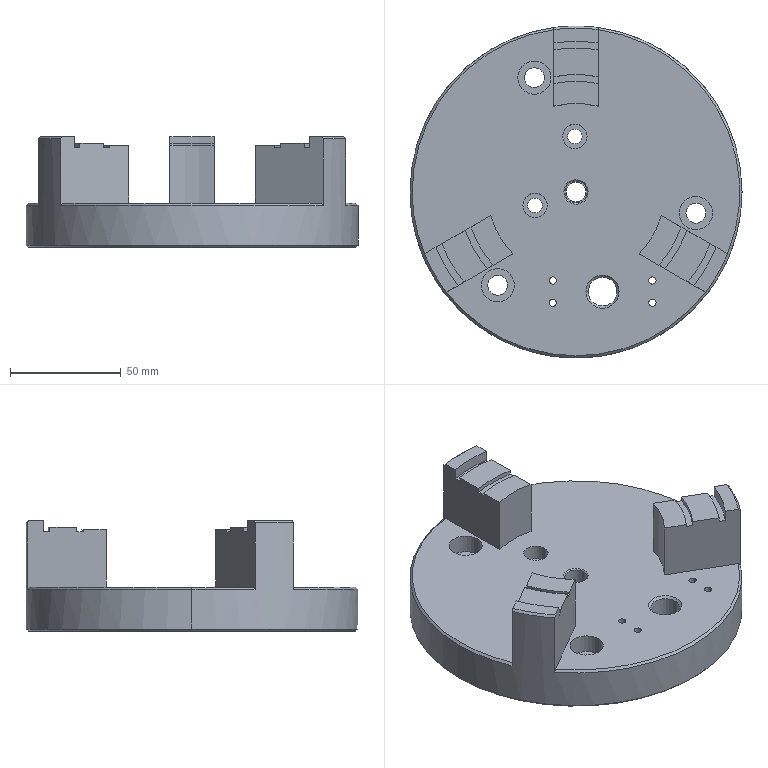Part | STEP file | Shim selection fixture body | 1 solid | 95 faces | box 150 x 150 x 50 mm | volume 396055 mm3 | cylinder 51 | plane 29 | cone 15 | commonest cylinder face diameters 3.3 x8 9 x8 15 x6 6.6 x4 11 x4 80 x3